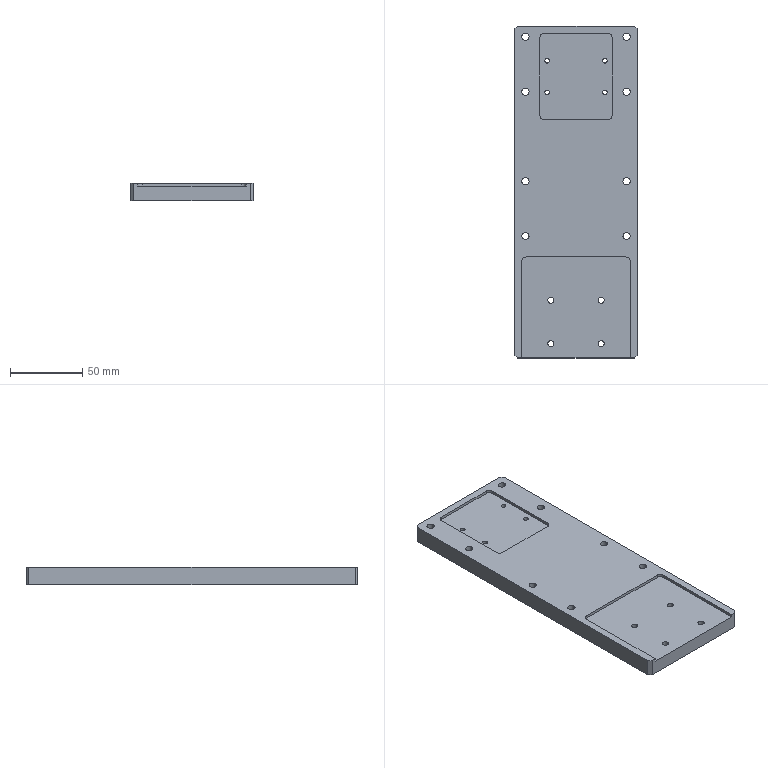Part | SolidWorks | features HoleWzd 3, Chamfer 1, Extrusion 1, ICE 1 | 1 solid | 57 faces | box 85 x 230 x 12 mm | volume 215246 mm3 | cylinder 38 | plane 19 | commonest cylinder face diameters 5 x16 3.3 x8 4.2 x8 6 x6